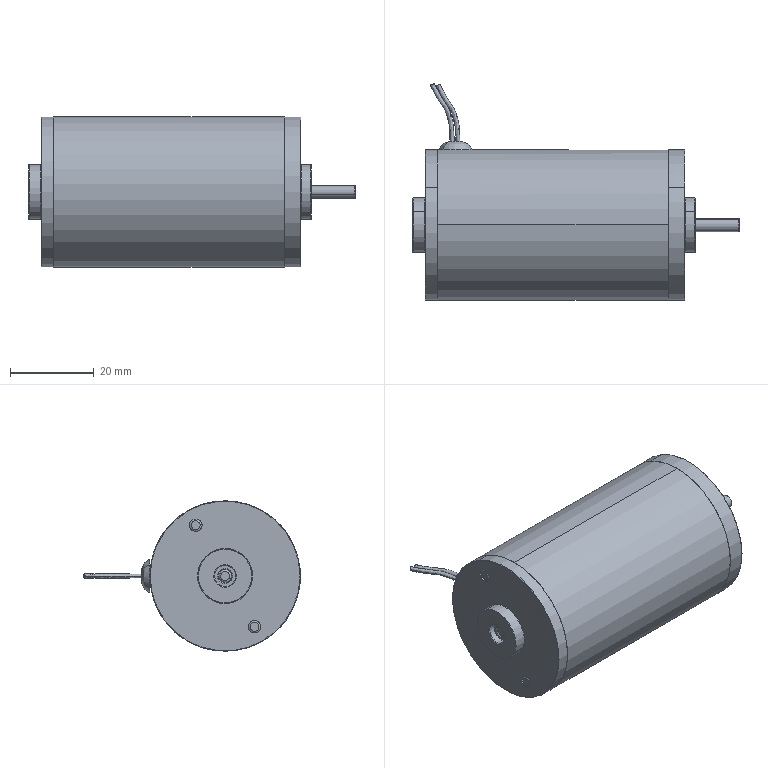Part | SolidWorks | 20 solids | 2076 faces | box 78 x 51.825 x 36 mm | volume 33870 mm3 | cylinder 1061 | cone 488 | torus 277 | plane 220 | sphere 22 | spline 8 | commonest cylinder face diameters 1 x852 1.179 x28 0.589 x16 2 x14 3 x14 5.5 x12